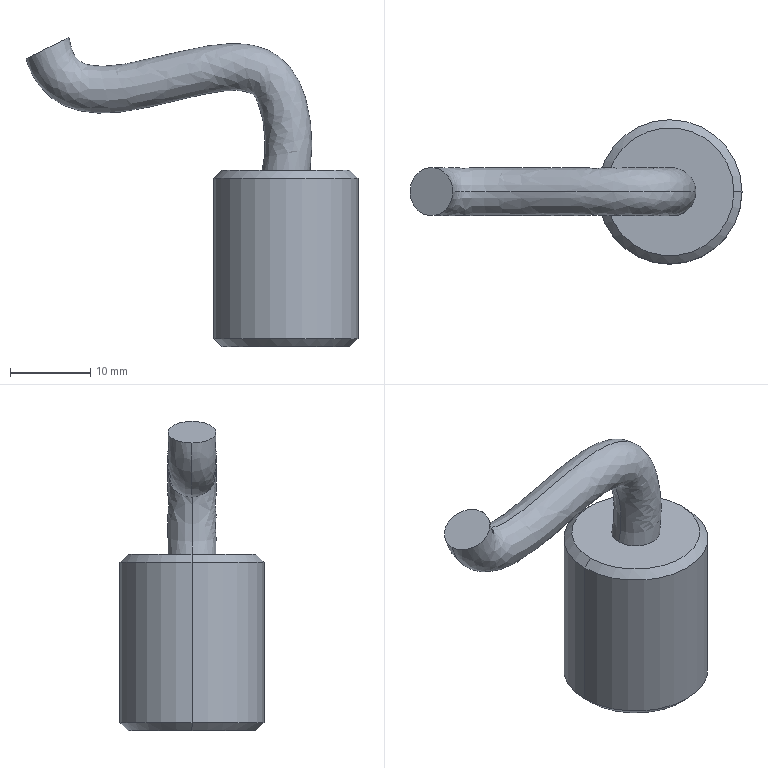Part | SolidWorks | features Chamfer 1, Extrusion 1, Sweep 1 | 1 solid | 11 faces | box 41.439 x 18 x 38.614 mm | volume 6724 mm3 | cone 4 | plane 3 | spline 2 | cylinder 2 | commonest cylinder face diameters 18 x2
STEP:
#1=CARTESIAN_POINT('',(3.,0.,11.));
#2=VERTEX_POINT('',#1);
#3=CARTESIAN_POINT('',(-3.,0.,11.));
#4=VERTEX_POINT('',#3);
#5=CARTESIAN_POINT('',(0.,0.,11.));
#6=DIRECTION('',(0.,0.,1.));
#7=DIRECTION('',(1.,0.,0.));
#8=AXIS2_PLACEMENT_3D('',#5,#6,#7);
#9=CIRCLE('',#8,3.);
#10=EDGE_CURVE('',#2,#4,#9,.T.);
#11=ORIENTED_EDGE('',*,*,#10,.T.);
#12=CARTESIAN_POINT('',(-32.439,0.,24.904));
#13=VERTEX_POINT('',#12);
#14=CARTESIAN_POINT('',(-3.,0.,11.));
#15=CARTESIAN_POINT('',(-2.85,0.,11.421));
#16=CARTESIAN_POINT('',(-2.631,0.,12.544));
#17=CARTESIAN_POINT('',(-2.558,0.,14.898));
#18=CARTESIAN_POINT('',(-2.81,0.,17.258));
#19=CARTESIAN_POINT('',(-3.262,0.,18.888));
#20=CARTESIAN_POINT('',(-3.573,0.,19.598));
#21=CARTESIAN_POINT('',(-3.703,0.,19.921));
#22=CARTESIAN_POINT('',(-3.832,0.,20.182));
#23=CARTESIAN_POINT('',(-4.134,0.,20.515));
#24=CARTESIAN_POINT('',(-5.011,0.,20.928));
#25=CARTESIAN_POINT('',(-6.881,0.,21.08));
#26=CARTESIAN_POINT('',(-10.217,0.,20.577));
#27=CARTESIAN_POINT('',(-14.463,0.,19.502));
#28=CARTESIAN_POINT('',(-19.332,0.,18.356));
#29=CARTESIAN_POINT('',(-23.167,0.,17.996));
#30=CARTESIAN_POINT('',(-25.981,0.,18.439));
#31=CARTESIAN_POINT('',(-27.667,0.,19.007));
#32=CARTESIAN_POINT('',(-29.133,0.,19.872));
#33=CARTESIAN_POINT('',(-30.31,0.,20.94));
#34=CARTESIAN_POINT('',(-31.207,0.,22.094));
#35=CARTESIAN_POINT('',(-31.928,0.,23.416));
#36=CARTESIAN_POINT('',(-32.28,0.,24.389));
#37=CARTESIAN_POINT('',(-32.439,0.,24.904));
#38=B_SPLINE_CURVE_WITH_KNOTS('',3,(#14,#15,#16,#17,#18,#19,#20,#21,#22,#23,#24,#25,#26,#27,#28,#29,#30,#31,#32,#33,#34,#35,#36,#37),.UNSPECIFIED.,.F.,.F.,(4,1,1,1,1,1,1,1,1,1,1,1,1,1,1,1,1,1,1,1,1,4),(0.,0.0625,0.125,0.1875,0.25,0.2852,0.2991,0.3203,0.3555,0.3906,0.4609,0.5313,0.625,0.7188,0.8125,0.8437,0.875,0.9063,0.9297,0.9531,0.9766,1.),.UNSPECIFIED.);
#39=EDGE_CURVE('',#4,#13,#38,.T.);
#40=ORIENTED_EDGE('',*,*,#39,.T.);
#41=CARTESIAN_POINT('',(-27.086,0.,27.614));
#42=VERTEX_POINT('',#41);
#43=CARTESIAN_POINT('',(-29.762,0.,26.259));
#44=DIRECTION('',(0.4517,0.,-0.8922));
#45=DIRECTION('',(-0.8922,0.,-0.4517));
#46=AXIS2_PLACEMENT_3D('',#43,#44,#45);
#47=CIRCLE('',#46,3.);
#48=EDGE_CURVE('',#13,#42,#47,.T.);
#49=ORIENTED_EDGE('',*,*,#48,.T.);
#50=CARTESIAN_POINT('',(3.,0.,11.));
#51=CARTESIAN_POINT('',(3.127,0.,11.782));
#52=CARTESIAN_POINT('',(3.302,0.,13.63));
#53=CARTESIAN_POINT('',(3.187,0.,16.671));
#54=CARTESIAN_POINT('',(2.615,0.,19.895));
#55=CARTESIAN_POINT('',(1.565,0.,22.549));
#56=CARTESIAN_POINT('',(0.3239,0.,24.212));
#57=CARTESIAN_POINT('',(-0.6963,0.,25.127));
#58=CARTESIAN_POINT('',(-1.844,0.,25.902));
#59=CARTESIAN_POINT('',(-3.45,0.,26.527));
#60=CARTESIAN_POINT('',(-5.923,0.,26.93));
#61=CARTESIAN_POINT('',(-8.914,0.,26.745));
#62=CARTESIAN_POINT('',(-12.881,0.,25.959));
#63=CARTESIAN_POINT('',(-17.232,0.,24.825));
#64=CARTESIAN_POINT('',(-21.638,0.,23.911));
#65=CARTESIAN_POINT('',(-24.307,0.,23.981));
#66=CARTESIAN_POINT('',(-25.501,0.,24.453));
#67=CARTESIAN_POINT('',(-25.999,0.,24.819));
#68=CARTESIAN_POINT('',(-26.304,0.,25.21));
#69=CARTESIAN_POINT('',(-26.531,0.,25.637));
#70=CARTESIAN_POINT('',(-26.728,0.,26.122));
#71=CARTESIAN_POINT('',(-26.917,0.,26.754));
#72=CARTESIAN_POINT('',(-27.041,0.,27.308));
#73=CARTESIAN_POINT('',(-27.086,0.,27.614));
#74=B_SPLINE_CURVE_WITH_KNOTS('',3,(#50,#51,#52,#53,#54,#55,#56,#57,#58,#59,#60,#61,#62,#63,#64,#65,#66,#67,#68,#69,#70,#71,#72,#73),.UNSPECIFIED.,.F.,.F.,(4,1,1,1,1,1,1,1,1,1,1,1,1,1,1,1,1,1,1,1,1,4),(0.,0.0625,0.125,0.1875,0.25,0.2852,0.2991,0.3203,0.3555,0.3906,0.4609,0.5313,0.625,0.7188,0.8125,0.8437,0.875,0.9063,0.9297,0.9531,0.9766,1.),.UNSPECIFIED.);
#75=EDGE_CURVE('',#2,#42,#74,.T.);
#76=ORIENTED_EDGE('',*,*,#75,.F.);
#77=EDGE_LOOP('',(#11,#40,#49,#76));
#78=FACE_OUTER_BOUND('',#77,.T.);
#79=CARTESIAN_POINT('',(3.,0.,11.));
#80=CARTESIAN_POINT('',(3.127,0.,11.782));
#81=CARTESIAN_POINT('',(3.302,0.,13.63));
#82=CARTESIAN_POINT('',(3.187,0.,16.671));
#83=CARTESIAN_POINT('',(2.615,0.,19.895));
#84=CARTESIAN_POINT('',(1.565,0.,22.549));
#85=CARTESIAN_POINT('',(0.3239,0.,24.212));
#86=CARTESIAN_POINT('',(-0.6963,0.,25.127));
#87=CARTESIAN_POINT('',(-1.844,0.,25.902));
#88=CARTESIAN_POINT('',(-3.45,0.,26.527));
#89=CARTESIAN_POINT('',(-5.923,0.,26.93));
#90=CARTESIAN_POINT('',(-8.914,0.,26.745));
#91=CARTESIAN_POINT('',(-12.881,0.,25.959));
#92=CARTESIAN_POINT('',(-17.232,0.,24.825));
#93=CARTESIAN_POINT('',(-21.638,0.,23.911));
#94=CARTESIAN_POINT('',(-24.307,0.,23.981));
#95=CARTESIAN_POINT('',(-25.501,0.,24.453));
#96=CARTESIAN_POINT('',(-25.999,0.,24.819));
#97=CARTESIAN_POINT('',(-26.304,0.,25.21));
#98=CARTESIAN_POINT('',(-26.531,0.,25.637));
#99=CARTESIAN_POINT('',(-26.728,0.,26.122));
#100=CARTESIAN_POINT('',(-26.917,0.,26.754));
#101=CARTESIAN_POINT('',(-27.041,0.,27.308));
#102=CARTESIAN_POINT('',(-27.086,0.,27.614));
#103=CARTESIAN_POINT('',(3.,6.,11.));
#104=CARTESIAN_POINT('',(3.127,6.,11.782));
#105=CARTESIAN_POINT('',(3.302,6.,13.63));
#106=CARTESIAN_POINT('',(3.187,6.,16.671));
#107=CARTESIAN_POINT('',(2.615,6.,19.895));
#108=CARTESIAN_POINT('',(1.565,6.,22.549));
#109=CARTESIAN_POINT('',(0.3239,6.,24.212));
#110=CARTESIAN_POINT('',(-0.6963,6.,25.127));
#111=CARTESIAN_POINT('',(-1.844,6.,25.902));
#112=CARTESIAN_POINT('',(-3.45,6.,26.527));
#113=CARTESIAN_POINT('',(-5.923,6.,26.93));
#114=CARTESIAN_POINT('',(-8.914,6.,26.745));
#115=CARTESIAN_POINT('',(-12.881,6.,25.959));
#116=CARTESIAN_POINT('',(-17.232,6.,24.825));
#117=CARTESIAN_POINT('',(-21.638,6.,23.911));
#118=CARTESIAN_POINT('',(-24.307,6.,23.981));
#119=CARTESIAN_POINT('',(-25.501,6.,24.453));
#120=CARTESIAN_POINT('',(-25.999,6.,24.819));
#121=CARTESIAN_POINT('',(-26.304,6.,25.21));
#122=CARTESIAN_POINT('',(-26.531,6.,25.637));
#123=CARTESIAN_POINT('',(-26.728,6.,26.122));
#124=CARTESIAN_POINT('',(-26.917,6.,26.754));
#125=CARTESIAN_POINT('',(-27.041,6.,27.308));
#126=CARTESIAN_POINT('',(-27.086,6.,27.614));
#127=CARTESIAN_POINT('',(-3.,6.,11.));
#128=CARTESIAN_POINT('',(-2.85,6.,11.421));
#129=CARTESIAN_POINT('',(-2.631,6.,12.544));
#130=CARTESIAN_POINT('',(-2.558,6.,14.898));
#131=CARTESIAN_POINT('',(-2.81,6.,17.258));
#132=CARTESIAN_POINT('',(-3.262,6.,18.888));
#133=CARTESIAN_POINT('',(-3.573,6.,19.598));
#134=CARTESIAN_POINT('',(-3.703,6.,19.921));
#135=CARTESIAN_POINT('',(-3.832,6.,20.182));
#136=CARTESIAN_POINT('',(-4.134,6.,20.515));
#137=CARTESIAN_POINT('',(-5.011,6.,20.928));
#138=CARTESIAN_POINT('',(-6.881,6.,21.08));
#139=CARTESIAN_POINT('',(-10.217,6.,20.577));
#140=CARTESIAN_POINT('',(-14.463,6.,19.502));
#141=CARTESIAN_POINT('',(-19.332,6.,18.356));
#142=CARTESIAN_POINT('',(-23.167,6.,17.996));
#143=CARTESIAN_POINT('',(-25.981,6.,18.439));
#144=CARTESIAN_POINT('',(-27.667,6.,19.007));
#145=CARTESIAN_POINT('',(-29.133,6.,19.872));
#146=CARTESIAN_POINT('',(-30.31,6.,20.94));
#147=CARTESIAN_POINT('',(-31.207,6.,22.094));
#148=CARTESIAN_POINT('',(-31.928,6.,23.416));
#149=CARTESIAN_POINT('',(-32.28,6.,24.389));
#150=CARTESIAN_POINT('',(-32.439,6.,24.904));
#151=CARTESIAN_POINT('',(-3.,0.,11.));
#152=CARTESIAN_POINT('',(-2.85,0.,11.421));
#153=CARTESIAN_POINT('',(-2.631,0.,12.544));
#154=CARTESIAN_POINT('',(-2.558,0.,14.898));
#155=CARTESIAN_POINT('',(-2.81,0.,17.258));
#156=CARTESIAN_POINT('',(-3.262,0.,18.888));
#157=CARTESIAN_POINT('',(-3.573,0.,19.598));
#158=CARTESIAN_POINT('',(-3.703,0.,19.921));
#159=CARTESIAN_POINT('',(-3.832,0.,20.182));
#160=CARTESIAN_POINT('',(-4.134,0.,20.515));
#161=CARTESIAN_POINT('',(-5.011,0.,20.928));
#162=CARTESIAN_POINT('',(-6.881,0.,21.08));
#163=CARTESIAN_POINT('',(-10.217,0.,20.577));
#164=CARTESIAN_POINT('',(-14.463,0.,19.502));
#165=CARTESIAN_POINT('',(-19.332,0.,18.356));
#166=CARTESIAN_POINT('',(-23.167,0.,17.996));
#167=CARTESIAN_POINT('',(-25.981,0.,18.439));
#168=CARTESIAN_POINT('',(-27.667,0.,19.007));
#169=CARTESIAN_POINT('',(-29.133,0.,19.872));
#170=CARTESIAN_POINT('',(-30.31,0.,20.94));
#171=CARTESIAN_POINT('',(-31.207,0.,22.094));
#172=CARTESIAN_POINT('',(-31.928,0.,23.416));
#173=CARTESIAN_POINT('',(-32.28,0.,24.389));
#174=CARTESIAN_POINT('',(-32.439,0.,24.904));
#175=CARTESIAN_POINT('',(-3.,-6.,11.));
#176=CARTESIAN_POINT('',(-2.85,-6.,11.421));
#177=CARTESIAN_POINT('',(-2.631,-6.,12.544));
#178=CARTESIAN_POINT('',(-2.558,-6.,14.898));
#179=CARTESIAN_POINT('',(-2.81,-6.,17.258));
#180=CARTESIAN_POINT('',(-3.262,-6.,18.888));
#181=CARTESIAN_POINT('',(-3.573,-6.,19.598));
#182=CARTESIAN_POINT('',(-3.703,-6.,19.921));
#183=CARTESIAN_POINT('',(-3.832,-6.,20.182));
#184=CARTESIAN_POINT('',(-4.134,-6.,20.515));
#185=CARTESIAN_POINT('',(-5.011,-6.,20.928));
#186=CARTESIAN_POINT('',(-6.881,-6.,21.08));
#187=CARTESIAN_POINT('',(-10.217,-6.,20.577));
#188=CARTESIAN_POINT('',(-14.463,-6.,19.502));
#189=CARTESIAN_POINT('',(-19.332,-6.,18.356));
#190=CARTESIAN_POINT('',(-23.167,-6.,17.996));
#191=CARTESIAN_POINT('',(-25.981,-6.,18.439));
#192=CARTESIAN_POINT('',(-27.667,-6.,19.007));
#193=CARTESIAN_POINT('',(-29.133,-6.,19.872));
#194=CARTESIAN_POINT('',(-30.31,-6.,20.94));
#195=CARTESIAN_POINT('',(-31.207,-6.,22.094));
#196=CARTESIAN_POINT('',(-31.928,-6.,23.416));
#197=CARTESIAN_POINT('',(-32.28,-6.,24.389));
#198=CARTESIAN_POINT('',(-32.439,-6.,24.904));
#199=CARTESIAN_POINT('',(3.,-6.,11.));
#200=CARTESIAN_POINT('',(3.127,-6.,11.782));
#201=CARTESIAN_POINT('',(3.302,-6.,13.63));
#202=CARTESIAN_POINT('',(3.187,-6.,16.671));
#203=CARTESIAN_POINT('',(2.615,-6.,19.895));
#204=CARTESIAN_POINT('',(1.565,-6.,22.549));
#205=CARTESIAN_POINT('',(0.3239,-6.,24.212));
#206=CARTESIAN_POINT('',(-0.6963,-6.,25.127));
#207=CARTESIAN_POINT('',(-1.844,-6.,25.902));
#208=CARTESIAN_POINT('',(-3.45,-6.,26.527));
#209=CARTESIAN_POINT('',(-5.923,-6.,26.93));
#210=CARTESIAN_POINT('',(-8.914,-6.,26.745));
#211=CARTESIAN_POINT('',(-12.881,-6.,25.959));
#212=CARTESIAN_POINT('',(-17.232,-6.,24.825));
#213=CARTESIAN_POINT('',(-21.638,-6.,23.911));
#214=CARTESIAN_POINT('',(-24.307,-6.,23.981));
#215=CARTESIAN_POINT('',(-25.501,-6.,24.453));
#216=CARTESIAN_POINT('',(-25.999,-6.,24.819));
#217=CARTESIAN_POINT('',(-26.304,-6.,25.21));
#218=CARTESIAN_POINT('',(-26.531,-6.,25.637));
#219=CARTESIAN_POINT('',(-26.728,-6.,26.122));
#220=CARTESIAN_POINT('',(-26.917,-6.,26.754));
#221=CARTESIAN_POINT('',(-27.041,-6.,27.308));
#222=CARTESIAN_POINT('',(-27.086,-6.,27.614));
#223=CARTESIAN_POINT('',(3.,0.,11.));
#224=CARTESIAN_POINT('',(3.127,0.,11.782));
#225=CARTESIAN_POINT('',(3.302,0.,13.63));
#226=CARTESIAN_POINT('',(3.187,0.,16.671));
#227=CARTESIAN_POINT('',(2.615,0.,19.895));
#228=CARTESIAN_POINT('',(1.565,0.,22.549));
#229=CARTESIAN_POINT('',(0.3239,0.,24.212));
#230=CARTESIAN_POINT('',(-0.6963,0.,25.127));
#231=CARTESIAN_POINT('',(-1.844,0.,25.902));
#232=CARTESIAN_POINT('',(-3.45,0.,26.527));
#233=CARTESIAN_POINT('',(-5.923,0.,26.93));
#234=CARTESIAN_POINT('',(-8.914,0.,26.745));
#235=CARTESIAN_POINT('',(-12.881,0.,25.959));
#236=CARTESIAN_POINT('',(-17.232,0.,24.825));
#237=CARTESIAN_POINT('',(-21.638,0.,23.911));
#238=CARTESIAN_POINT('',(-24.307,0.,23.981));
#239=CARTESIAN_POINT('',(-25.501,0.,24.453));
#240=CARTESIAN_POINT('',(-25.999,0.,24.819));
#241=CARTESIAN_POINT('',(-26.304,0.,25.21));
#242=CARTESIAN_POINT('',(-26.531,0.,25.637));
#243=CARTESIAN_POINT('',(-26.728,0.,26.122));
#244=CARTESIAN_POINT('',(-26.917,0.,26.754));
#245=CARTESIAN_POINT('',(-27.041,0.,27.308));
#246=CARTESIAN_POINT('',(-27.086,0.,27.614));
#247=(BOUNDED_SURFACE()B_SPLINE_SURFACE(3,3,((#79,#80,#81,#82,#83,#84,#85,#86,#87,#88,#89,#90,#91,#92,#93,#94,#95,#96,#97,#98,#99,#100,#101,#102),(#103,#104,#105,#106,#107,#108,#109,#110,#111,#112,#113,#114,#115,#116,#117,#118,#119,#120,#121,#122,#123,#124,#125,#126),(#127,#128,#129,#130,#131,#132,#133,#134,#135,#136,#137,#138,#139,#140,#141,#142,#143,#144,#145,#146,#147,#148,#149,#150),(#151,#152,#153,#154,#155,#156,#157,#158,#159,#160,#161,#162,#163,#164,#165,#166,#167,#168,#169,#170,#171,#172,#173,#174),(#175,#176,#177,#178,#179,#180,#181,#182,#183,#184,#185,#186,#187,#188,#189,#190,#191,#192,#193,#194,#195,#196,#197,#198),(#199,#200,#201,#202,#203,#204,#205,#206,#207,#208,#209,#210,#211,#212,#213,#214,#215,#216,#217,#218,#219,#220,#221,#222),(#223,#224,#225,#226,#227,#228,#229,#230,#231,#232,#233,#234,#235,#236,#237,#238,#239,#240,#241,#242,#243,#244,#245,#246)),.UNSPECIFIED.,.T.,.F.,.T.)B_SPLINE_SURFACE_WITH_KNOTS((4,3,4),(4,1,1,1,1,1,1,1,1,1,1,1,1,1,1,1,1,1,1,1,1,4),(0.,0.5,1.),(0.,0.0625,0.125,0.1875,0.25,0.2852,0.2991,0.3203,0.3555,0.3906,0.4609,0.5313,0.625,0.7188,0.8125,0.8437,0.875,0.9063,0.9297,0.9531,0.9766,1.),.UNSPECIFIED.)GEOMETRIC_REPRESENTATION_ITEM()RATIONAL_B_SPLINE_SURFACE(((1.,1.,1.,1.,1.,1.,1.,1.,1.,1.,1.,1.,1.,1.,1.,1.,1.,1.,1.,1.,1.,1.,1.,1.),(0.3333,0.3333,0.3333,0.3333,0.3333,0.3333,0.3333,0.3333,0.3333,0.3333,0.3333,0.3333,0.3333,0.3333,0.3333,0.3333,0.3333,0.3333,0.3333,0.3333,0.3333,0.3333,0.3333,0.3333),(0.3333,0.3333,0.3333,0.3333,0.3333,0.3333,0.3333,0.3333,0.3333,0.3333,0.3333,0.3333,0.3333,0.3333,0.3333,0.3333,0.3333,0.3333,0.3333,0.3333,0.3333,0.3333,0.3333,0.3333),(1.,1.,1.,1.,1.,1.,1.,1.,1.,1.,1.,1.,1.,1.,1.,1.,1.,1.,1.,1.,1.,1.,1.,1.),(0.3333,0.3333,0.3333,0.3333,0.3333,0.3333,0.3333,0.3333,0.3333,0.3333,0.3333,0.3333,0.3333,0.3333,0.3333,0.3333,0.3333,0.3333,0.3333,0.3333,0.3333,0.3333,0.3333,0.3333),(0.3333,0.3333,0.3333,0.3333,0.3333,0.3333,0.3333,0.3333,0.3333,0.3333,0.3333,0.3333,0.3333,0.3333,0.3333,0.3333,0.3333,0.3333,0.3333,0.3333,0.3333,0.3333,0.3333,0.3333),(1.,1.,1.,1.,1.,1.,1.,1.,1.,1.,1.,1.,1.,1.,1.,1.,1.,1.,1.,1.,1.,1.,1.,1.)))REPRESENTATION_ITEM('')SURFACE());
#248=ADVANCED_FACE('',(#78),#247,.T.);
#249=CARTESIAN_POINT('',(8.,0.,11.));
#250=VERTEX_POINT('',#249);
#251=CARTESIAN_POINT('',(-8.,0.,11.));
#252=VERTEX_POINT('',#251);
#253=CARTESIAN_POINT('',(0.,0.,11.));
#254=DIRECTION('',(0.,0.,1.));
#255=DIRECTION('',(1.,0.,0.));
#256=AXIS2_PLACEMENT_3D('',#253,#254,#255);
#257=CIRCLE('',#256,8.);
#258=EDGE_CURVE('',#250,#252,#257,.T.);
#259=ORIENTED_EDGE('',*,*,#258,.F.);
#260=CARTESIAN_POINT('',(9.,0.,10.));
#261=VERTEX_POINT('',#260);
#262=CARTESIAN_POINT('',(8.,0.,11.));
#263=DIRECTION('',(0.7071,0.,-0.7071));
#264=VECTOR('',#263,1000.);
#265=LINE('',#262,#264);
#266=EDGE_CURVE('',#250,#261,#265,.T.);
#267=ORIENTED_EDGE('',*,*,#266,.T.);
#268=CARTESIAN_POINT('',(-9.,0.,10.));
#269=VERTEX_POINT('',#268);
#270=CARTESIAN_POINT('',(0.,0.,10.));
#271=DIRECTION('',(0.,0.,-1.));
#272=DIRECTION('',(1.,0.,0.));
#273=AXIS2_PLACEMENT_3D('',#270,#271,#272);
#274=CIRCLE('',#273,9.);
#275=EDGE_CURVE('',#269,#261,#274,.T.);
#276=ORIENTED_EDGE('',*,*,#275,.F.);
#277=CARTESIAN_POINT('',(-8.,0.,11.));
#278=DIRECTION('',(-0.7071,0.,-0.7071));
#279=VECTOR('',#278,1000.);
#280=LINE('',#277,#279);
#281=EDGE_CURVE('',#252,#269,#280,.T.);
#282=ORIENTED_EDGE('',*,*,#281,.F.);
#283=EDGE_LOOP('',(#259,#267,#276,#282));
#284=FACE_OUTER_BOUND('',#283,.T.);
#285=CARTESIAN_POINT('',(0.,0.,11.));
#286=DIRECTION('',(0.,0.,-1.));
#287=DIRECTION('',(-1.,0.,0.));
#288=AXIS2_PLACEMENT_3D('',#285,#286,#287);
#289=CONICAL_SURFACE('',#288,8.,0.7854);
#290=ADVANCED_FACE('',(#284),#289,.T.);
#291=CARTESIAN_POINT('',(-8.,0.,-11.));
#292=VERTEX_POINT('',#291);
#293=CARTESIAN_POINT('',(8.,0.,-11.));
#294=VERTEX_POINT('',#293);
#295=CARTESIAN_POINT('',(0.,0.,-11.));
#296=DIRECTION('',(0.,0.,-1.));
#297=DIRECTION('',(1.,0.,0.));
#298=AXIS2_PLACEMENT_3D('',#295,#296,#297);
#299=CIRCLE('',#298,8.);
#300=EDGE_CURVE('',#292,#294,#299,.T.);
#301=ORIENTED_EDGE('',*,*,#300,.F.);
#302=CARTESIAN_POINT('',(-9.,0.,-10.));
#303=VERTEX_POINT('',#302);
#304=CARTESIAN_POINT('',(-9.,0.,-10.));
#305=DIRECTION('',(-0.7071,0.,0.7071));
#306=VECTOR('',#305,1000.);
#307=LINE('',#304,#306);
#308=EDGE_CURVE('',#292,#303,#307,.T.);
#309=ORIENTED_EDGE('',*,*,#308,.T.);
#310=CARTESIAN_POINT('',(9.,0.,-10.));
#311=VERTEX_POINT('',#310);
#312=CARTESIAN_POINT('',(0.,0.,-10.));
#313=DIRECTION('',(0.,0.,1.));
#314=DIRECTION('',(1.,0.,0.));
#315=AXIS2_PLACEMENT_3D('',#312,#313,#314);
#316=CIRCLE('',#315,9.);
#317=EDGE_CURVE('',#311,#303,#316,.T.);
#318=ORIENTED_EDGE('',*,*,#317,.F.);
#319=CARTESIAN_POINT('',(9.,0.,-10.));
#320=DIRECTION('',(0.7071,0.,0.7071));
#321=VECTOR('',#320,1000.);
#322=LINE('',#319,#321);
#323=EDGE_CURVE('',#294,#311,#322,.T.);
#324=ORIENTED_EDGE('',*,*,#323,.F.);
#325=EDGE_LOOP('',(#301,#309,#318,#324));
#326=FACE_OUTER_BOUND('',#325,.T.);
#327=CARTESIAN_POINT('',(0.,0.,-10.));
#328=DIRECTION('',(0.,0.,1.));
#329=DIRECTION('',(1.,0.,0.));
#330=AXIS2_PLACEMENT_3D('',#327,#328,#329);
#331=CONICAL_SURFACE('',#330,9.,0.7854);
#332=ADVANCED_FACE('',(#326),#331,.T.);
#333=ORIENTED_EDGE('',*,*,#275,.T.);
#334=CARTESIAN_POINT('',(9.,0.,11.));
#335=DIRECTION('',(0.,0.,-1.));
#336=VECTOR('',#335,1000.);
#337=LINE('',#334,#336);
#338=EDGE_CURVE('',#261,#311,#337,.T.);
#339=ORIENTED_EDGE('',*,*,#338,.T.);
#340=ORIENTED_EDGE('',*,*,#317,.T.);
#341=CARTESIAN_POINT('',(-9.,0.,11.));
#342=DIRECTION('',(0.,0.,-1.));
#343=VECTOR('',#342,1000.);
#344=LINE('',#341,#343);
#345=EDGE_CURVE('',#269,#303,#344,.T.);
#346=ORIENTED_EDGE('',*,*,#345,.F.);
#347=EDGE_LOOP('',(#333,#339,#340,#346));
#348=FACE_OUTER_BOUND('',#347,.T.);
#349=CARTESIAN_POINT('',(0.,0.,11.));
#350=DIRECTION('',(0.,0.,-1.));
#351=DIRECTION('',(-1.,0.,0.));
#352=AXIS2_PLACEMENT_3D('',#349,#350,#351);
#353=CYLINDRICAL_SURFACE('',#352,9.);
#354=ADVANCED_FACE('',(#348),#353,.T.);
#355=ORIENTED_EDGE('',*,*,#338,.F.);
#356=CARTESIAN_POINT('',(0.,0.,10.));
#357=DIRECTION('',(0.,0.,-1.));
#358=DIRECTION('',(1.,0.,0.));
#359=AXIS2_PLACEMENT_3D('',#356,#357,#358);
#360=CIRCLE('',#359,9.);
#361=EDGE_CURVE('',#261,#269,#360,.T.);
#362=ORIENTED_EDGE('',*,*,#361,.T.);
#363=ORIENTED_EDGE('',*,*,#345,.T.);
#364=CARTESIAN_POINT('',(0.,0.,-10.));
#365=DIRECTION('',(0.,0.,1.));
#366=DIRECTION('',(1.,0.,0.));
#367=AXIS2_PLACEMENT_3D('',#364,#365,#366);
#368=CIRCLE('',#367,9.);
#369=EDGE_CURVE('',#303,#311,#368,.T.);
#370=ORIENTED_EDGE('',*,*,#369,.T.);
#371=EDGE_LOOP('',(#355,#362,#363,#370));
#372=FACE_OUTER_BOUND('',#371,.T.);
#373=CARTESIAN_POINT('',(0.,0.,11.));
#374=DIRECTION('',(0.,0.,-1.));
#375=DIRECTION('',(-1.,0.,0.));
#376=AXIS2_PLACEMENT_3D('',#373,#374,#375);
#377=CYLINDRICAL_SURFACE('',#376,9.);
#378=ADVANCED_FACE('',(#372),#377,.T.);
#379=ORIENTED_EDGE('',*,*,#10,.F.);
#380=CARTESIAN_POINT('',(0.,0.,11.));
#381=DIRECTION('',(0.,0.,1.));
#382=DIRECTION('',(1.,0.,0.));
#383=AXIS2_PLACEMENT_3D('',#380,#381,#382);
#384=CIRCLE('',#383,3.);
#385=EDGE_CURVE('',#4,#2,#384,.T.);
#386=ORIENTED_EDGE('',*,*,#385,.F.);
#387=EDGE_LOOP('',(#379,#386));
#388=FACE_BOUND('',#387,.T.);
#389=CARTESIAN_POINT('',(0.,0.,11.));
#390=DIRECTION('',(0.,0.,1.));
#391=DIRECTION('',(1.,0.,0.));
#392=AXIS2_PLACEMENT_3D('',#389,#390,#391);
#393=CIRCLE('',#392,8.);
#394=EDGE_CURVE('',#252,#250,#393,.T.);
#395=ORIENTED_EDGE('',*,*,#394,.T.);
#396=ORIENTED_EDGE('',*,*,#258,.T.);
#397=EDGE_LOOP('',(#395,#396));
#398=FACE_OUTER_BOUND('',#397,.T.);
#399=CARTESIAN_POINT('',(0.,0.,11.));
#400=DIRECTION('',(0.,0.,1.));
#401=DIRECTION('',(1.,0.,0.));
#402=AXIS2_PLACEMENT_3D('',#399,#400,#401);
#403=PLANE('',#402);
#404=ADVANCED_FACE('',(#388,#398),#403,.T.);
#405=CARTESIAN_POINT('',(0.,0.,-11.));
#406=DIRECTION('',(0.,0.,-1.));
#407=DIRECTION('',(1.,0.,0.));
#408=AXIS2_PLACEMENT_3D('',#405,#406,#407);
#409=CIRCLE('',#408,8.);
#410=EDGE_CURVE('',#294,#292,#409,.T.);
#411=ORIENTED_EDGE('',*,*,#410,.T.);
#412=ORIENTED_EDGE('',*,*,#300,.T.);
#413=EDGE_LOOP('',(#411,#412));
#414=FACE_OUTER_BOUND('',#413,.T.);
#415=CARTESIAN_POINT('',(0.,0.,-11.));
#416=DIRECTION('',(0.,0.,1.));
#417=DIRECTION('',(1.,0.,0.));
#418=AXIS2_PLACEMENT_3D('',#415,#416,#417);
#419=PLANE('',#418);
#420=ADVANCED_FACE('',(#414),#419,.F.);
#421=ORIENTED_EDGE('',*,*,#308,.F.);
#422=ORIENTED_EDGE('',*,*,#410,.F.);
#423=ORIENTED_EDGE('',*,*,#323,.T.);
#424=ORIENTED_EDGE('',*,*,#369,.F.);
#425=EDGE_LOOP('',(#421,#422,#423,#424));
#426=FACE_OUTER_BOUND('',#425,.T.);
#427=CARTESIAN_POINT('',(0.,0.,-10.));
#428=DIRECTION('',(0.,0.,1.));
#429=DIRECTION('',(1.,0.,0.));
#430=AXIS2_PLACEMENT_3D('',#427,#428,#429);
#431=CONICAL_SURFACE('',#430,9.,0.7854);
#432=ADVANCED_FACE('',(#426),#431,.T.);
#433=ORIENTED_EDGE('',*,*,#266,.F.);
#434=ORIENTED_EDGE('',*,*,#394,.F.);
#435=ORIENTED_EDGE('',*,*,#281,.T.);
#436=ORIENTED_EDGE('',*,*,#361,.F.);
#437=EDGE_LOOP('',(#433,#434,#435,#436));
#438=FACE_OUTER_BOUND('',#437,.T.);
#439=CARTESIAN_POINT('',(0.,0.,11.));
#440=DIRECTION('',(0.,0.,-1.));
#441=DIRECTION('',(-1.,0.,0.));
#442=AXIS2_PLACEMENT_3D('',#439,#440,#441);
#443=CONICAL_SURFACE('',#442,8.,0.7854);
#444=ADVANCED_FACE('',(#438),#443,.T.);
#445=ORIENTED_EDGE('',*,*,#39,.F.);
#446=ORIENTED_EDGE('',*,*,#385,.T.);
#447=ORIENTED_EDGE('',*,*,#75,.T.);
#448=CARTESIAN_POINT('',(-29.762,0.,26.259));
#449=DIRECTION('',(0.4517,0.,-0.8922));
#450=DIRECTION('',(-0.8922,0.,-0.4517));
#451=AXIS2_PLACEMENT_3D('',#448,#449,#450);
#452=CIRCLE('',#451,3.);
#453=EDGE_CURVE('',#42,#13,#452,.T.);
#454=ORIENTED_EDGE('',*,*,#453,.T.);
#455=EDGE_LOOP('',(#445,#446,#447,#454));
#456=FACE_OUTER_BOUND('',#455,.T.);
#457=CARTESIAN_POINT('',(3.,0.,11.));
#458=CARTESIAN_POINT('',(3.127,0.,11.782));
#459=CARTESIAN_POINT('',(3.302,0.,13.63));
#460=CARTESIAN_POINT('',(3.187,0.,16.671));
#461=CARTESIAN_POINT('',(2.615,0.,19.895));
#462=CARTESIAN_POINT('',(1.565,0.,22.549));
#463=CARTESIAN_POINT('',(0.3239,0.,24.212));
#464=CARTESIAN_POINT('',(-0.6963,0.,25.127));
#465=CARTESIAN_POINT('',(-1.844,0.,25.902));
#466=CARTESIAN_POINT('',(-3.45,0.,26.527));
#467=CARTESIAN_POINT('',(-5.923,0.,26.93));
#468=CARTESIAN_POINT('',(-8.914,0.,26.745));
#469=CARTESIAN_POINT('',(-12.881,0.,25.959));
#470=CARTESIAN_POINT('',(-17.232,0.,24.825));
#471=CARTESIAN_POINT('',(-21.638,0.,23.911));
#472=CARTESIAN_POINT('',(-24.307,0.,23.981));
#473=CARTESIAN_POINT('',(-25.501,0.,24.453));
#474=CARTESIAN_POINT('',(-25.999,0.,24.819));
#475=CARTESIAN_POINT('',(-26.304,0.,25.21));
#476=CARTESIAN_POINT('',(-26.531,0.,25.637));
#477=CARTESIAN_POINT('',(-26.728,0.,26.122));
#478=CARTESIAN_POINT('',(-26.917,0.,26.754));
#479=CARTESIAN_POINT('',(-27.041,0.,27.308));
#480=CARTESIAN_POINT('',(-27.086,0.,27.614));
#481=CARTESIAN_POINT('',(3.,6.,11.));
#482=CARTESIAN_POINT('',(3.127,6.,11.782));
#483=CARTESIAN_POINT('',(3.302,6.,13.63));
#484=CARTESIAN_POINT('',(3.187,6.,16.671));
#485=CARTESIAN_POINT('',(2.615,6.,19.895));
#486=CARTESIAN_POINT('',(1.565,6.,22.549));
#487=CARTESIAN_POINT('',(0.3239,6.,24.212));
#488=CARTESIAN_POINT('',(-0.6963,6.,25.127));
#489=CARTESIAN_POINT('',(-1.844,6.,25.902));
#490=CARTESIAN_POINT('',(-3.45,6.,26.527));
#491=CARTESIAN_POINT('',(-5.923,6.,26.93));
#492=CARTESIAN_POINT('',(-8.914,6.,26.745));
#493=CARTESIAN_POINT('',(-12.881,6.,25.959));
#494=CARTESIAN_POINT('',(-17.232,6.,24.825));
#495=CARTESIAN_POINT('',(-21.638,6.,23.911));
#496=CARTESIAN_POINT('',(-24.307,6.,23.981));
#497=CARTESIAN_POINT('',(-25.501,6.,24.453));
#498=CARTESIAN_POINT('',(-25.999,6.,24.819));
#499=CARTESIAN_POINT('',(-26.304,6.,25.21));
#500=CARTESIAN_POINT('',(-26.531,6.,25.637));
#501=CARTESIAN_POINT('',(-26.728,6.,26.122));
#502=CARTESIAN_POINT('',(-26.917,6.,26.754));
#503=CARTESIAN_POINT('',(-27.041,6.,27.308));
#504=CARTESIAN_POINT('',(-27.086,6.,27.614));
#505=CARTESIAN_POINT('',(-3.,6.,11.));
#506=CARTESIAN_POINT('',(-2.85,6.,11.421));
#507=CARTESIAN_POINT('',(-2.631,6.,12.544));
#508=CARTESIAN_POINT('',(-2.558,6.,14.898));
#509=CARTESIAN_POINT('',(-2.81,6.,17.258));
#510=CARTESIAN_POINT('',(-3.262,6.,18.888));
#511=CARTESIAN_POINT('',(-3.573,6.,19.598));
#512=CARTESIAN_POINT('',(-3.703,6.,19.921));
#513=CARTESIAN_POINT('',(-3.832,6.,20.182));
#514=CARTESIAN_POINT('',(-4.134,6.,20.515));
#515=CARTESIAN_POINT('',(-5.011,6.,20.928));
#516=CARTESIAN_POINT('',(-6.881,6.,21.08));
#517=CARTESIAN_POINT('',(-10.217,6.,20.577));
#518=CARTESIAN_POINT('',(-14.463,6.,19.502));
#519=CARTESIAN_POINT('',(-19.332,6.,18.356));
#520=CARTESIAN_POINT('',(-23.167,6.,17.996));
#521=CARTESIAN_POINT('',(-25.981,6.,18.439));
#522=CARTESIAN_POINT('',(-27.667,6.,19.007));
#523=CARTESIAN_POINT('',(-29.133,6.,19.872));
#524=CARTESIAN_POINT('',(-30.31,6.,20.94));
#525=CARTESIAN_POINT('',(-31.207,6.,22.094));
#526=CARTESIAN_POINT('',(-31.928,6.,23.416));
#527=CARTESIAN_POINT('',(-32.28,6.,24.389));
#528=CARTESIAN_POINT('',(-32.439,6.,24.904));
#529=CARTESIAN_POINT('',(-3.,0.,11.));
#530=CARTESIAN_POINT('',(-2.85,0.,11.421));
#531=CARTESIAN_POINT('',(-2.631,0.,12.544));
#532=CARTESIAN_POINT('',(-2.558,0.,14.898));
#533=CARTESIAN_POINT('',(-2.81,0.,17.258));
#534=CARTESIAN_POINT('',(-3.262,0.,18.888));
#535=CARTESIAN_POINT('',(-3.573,0.,19.598));
#536=CARTESIAN_POINT('',(-3.703,0.,19.921));
#537=CARTESIAN_POINT('',(-3.832,0.,20.182));
#538=CARTESIAN_POINT('',(-4.134,0.,20.515));
#539=CARTESIAN_POINT('',(-5.011,0.,20.928));
#540=CARTESIAN_POINT('',(-6.881,0.,21.08));
#541=CARTESIAN_POINT('',(-10.217,0.,20.577));
#542=CARTESIAN_POINT('',(-14.463,0.,19.502));
#543=CARTESIAN_POINT('',(-19.332,0.,18.356));
#544=CARTESIAN_POINT('',(-23.167,0.,17.996));
#545=CARTESIAN_POINT('',(-25.981,0.,18.439));
#546=CARTESIAN_POINT('',(-27.667,0.,19.007));
#547=CARTESIAN_POINT('',(-29.133,0.,19.872));
#548=CARTESIAN_POINT('',(-30.31,0.,20.94));
#549=CARTESIAN_POINT('',(-31.207,0.,22.094));
#550=CARTESIAN_POINT('',(-31.928,0.,23.416));
#551=CARTESIAN_POINT('',(-32.28,0.,24.389));
#552=CARTESIAN_POINT('',(-32.439,0.,24.904));
#553=CARTESIAN_POINT('',(-3.,-6.,11.));
#554=CARTESIAN_POINT('',(-2.85,-6.,11.421));
#555=CARTESIAN_POINT('',(-2.631,-6.,12.544));
#556=CARTESIAN_POINT('',(-2.558,-6.,14.898));
#557=CARTESIAN_POINT('',(-2.81,-6.,17.258));
#558=CARTESIAN_POINT('',(-3.262,-6.,18.888));
#559=CARTESIAN_POINT('',(-3.573,-6.,19.598));
#560=CARTESIAN_POINT('',(-3.703,-6.,19.921));
#561=CARTESIAN_POINT('',(-3.832,-6.,20.182));
#562=CARTESIAN_POINT('',(-4.134,-6.,20.515));
#563=CARTESIAN_POINT('',(-5.011,-6.,20.928));
#564=CARTESIAN_POINT('',(-6.881,-6.,21.08));
#565=CARTESIAN_POINT('',(-10.217,-6.,20.577));
#566=CARTESIAN_POINT('',(-14.463,-6.,19.502));
#567=CARTESIAN_POINT('',(-19.332,-6.,18.356));
#568=CARTESIAN_POINT('',(-23.167,-6.,17.996));
#569=CARTESIAN_POINT('',(-25.981,-6.,18.439));
#570=CARTESIAN_POINT('',(-27.667,-6.,19.007));
#571=CARTESIAN_POINT('',(-29.133,-6.,19.872));
#572=CARTESIAN_POINT('',(-30.31,-6.,20.94));
#573=CARTESIAN_POINT('',(-31.207,-6.,22.094));
#574=CARTESIAN_POINT('',(-31.928,-6.,23.416));
#575=CARTESIAN_POINT('',(-32.28,-6.,24.389));
#576=CARTESIAN_POINT('',(-32.439,-6.,24.904));
#577=CARTESIAN_POINT('',(3.,-6.,11.));
#578=CARTESIAN_POINT('',(3.127,-6.,11.782));
#579=CARTESIAN_POINT('',(3.302,-6.,13.63));
#580=CARTESIAN_POINT('',(3.187,-6.,16.671));
#581=CARTESIAN_POINT('',(2.615,-6.,19.895));
#582=CARTESIAN_POINT('',(1.565,-6.,22.549));
#583=CARTESIAN_POINT('',(0.3239,-6.,24.212));
#584=CARTESIAN_POINT('',(-0.6963,-6.,25.127));
#585=CARTESIAN_POINT('',(-1.844,-6.,25.902));
#586=CARTESIAN_POINT('',(-3.45,-6.,26.527));
#587=CARTESIAN_POINT('',(-5.923,-6.,26.93));
#588=CARTESIAN_POINT('',(-8.914,-6.,26.745));
#589=CARTESIAN_POINT('',(-12.881,-6.,25.959));
#590=CARTESIAN_POINT('',(-17.232,-6.,24.825));
#591=CARTESIAN_POINT('',(-21.638,-6.,23.911));
#592=CARTESIAN_POINT('',(-24.307,-6.,23.981));
#593=CARTESIAN_POINT('',(-25.501,-6.,24.453));
#594=CARTESIAN_POINT('',(-25.999,-6.,24.819));
#595=CARTESIAN_POINT('',(-26.304,-6.,25.21));
#596=CARTESIAN_POINT('',(-26.531,-6.,25.637));
#597=CARTESIAN_POINT('',(-26.728,-6.,26.122));
#598=CARTESIAN_POINT('',(-26.917,-6.,26.754));
#599=CARTESIAN_POINT('',(-27.041,-6.,27.308));
#600=CARTESIAN_POINT('',(-27.086,-6.,27.614));
#601=CARTESIAN_POINT('',(3.,0.,11.));
#602=CARTESIAN_POINT('',(3.127,0.,11.782));
#603=CARTESIAN_POINT('',(3.302,0.,13.63));
#604=CARTESIAN_POINT('',(3.187,0.,16.671));
#605=CARTESIAN_POINT('',(2.615,0.,19.895));
#606=CARTESIAN_POINT('',(1.565,0.,22.549));
#607=CARTESIAN_POINT('',(0.3239,0.,24.212));
#608=CARTESIAN_POINT('',(-0.6963,0.,25.127));
#609=CARTESIAN_POINT('',(-1.844,0.,25.902));
#610=CARTESIAN_POINT('',(-3.45,0.,26.527));
#611=CARTESIAN_POINT('',(-5.923,0.,26.93));
#612=CARTESIAN_POINT('',(-8.914,0.,26.745));
#613=CARTESIAN_POINT('',(-12.881,0.,25.959));
#614=CARTESIAN_POINT('',(-17.232,0.,24.825));
#615=CARTESIAN_POINT('',(-21.638,0.,23.911));
#616=CARTESIAN_POINT('',(-24.307,0.,23.981));
#617=CARTESIAN_POINT('',(-25.501,0.,24.453));
#618=CARTESIAN_POINT('',(-25.999,0.,24.819));
#619=CARTESIAN_POINT('',(-26.304,0.,25.21));
#620=CARTESIAN_POINT('',(-26.531,0.,25.637));
#621=CARTESIAN_POINT('',(-26.728,0.,26.122));
#622=CARTESIAN_POINT('',(-26.917,0.,26.754));
#623=CARTESIAN_POINT('',(-27.041,0.,27.308));
#624=CARTESIAN_POINT('',(-27.086,0.,27.614));
#625=(BOUNDED_SURFACE()B_SPLINE_SURFACE(3,3,((#457,#458,#459,#460,#461,#462,#463,#464,#465,#466,#467,#468,#469,#470,#471,#472,#473,#474,#475,#476,#477,#478,#479,#480),(#481,#482,#483,#484,#485,#486,#487,#488,#489,#490,#491,#492,#493,#494,#495,#496,#497,#498,#499,#500,#501,#502,#503,#504),(#505,#506,#507,#508,#509,#510,#511,#512,#513,#514,#515,#516,#517,#518,#519,#520,#521,#522,#523,#524,#525,#526,#527,#528),(#529,#530,#531,#532,#533,#534,#535,#536,#537,#538,#539,#540,#541,#542,#543,#544,#545,#546,#547,#548,#549,#550,#551,#552),(#553,#554,#555,#556,#557,#558,#559,#560,#561,#562,#563,#564,#565,#566,#567,#568,#569,#570,#571,#572,#573,#574,#575,#576),(#577,#578,#579,#580,#581,#582,#583,#584,#585,#586,#587,#588,#589,#590,#591,#592,#593,#594,#595,#596,#597,#598,#599,#600),(#601,#602,#603,#604,#605,#606,#607,#608,#609,#610,#611,#612,#613,#614,#615,#616,#617,#618,#619,#620,#621,#622,#623,#624)),.UNSPECIFIED.,.T.,.F.,.F.)B_SPLINE_SURFACE_WITH_KNOTS((4,3,4),(4,1,1,1,1,1,1,1,1,1,1,1,1,1,1,1,1,1,1,1,1,4),(0.,0.5,1.),(0.,0.0625,0.125,0.1875,0.25,0.2852,0.2991,0.3203,0.3555,0.3906,0.4609,0.5313,0.625,0.7188,0.8125,0.8437,0.875,0.9063,0.9297,0.9531,0.9766,1.),.UNSPECIFIED.)GEOMETRIC_REPRESENTATION_ITEM()RATIONAL_B_SPLINE_SURFACE(((1.,1.,1.,1.,1.,1.,1.,1.,1.,1.,1.,1.,1.,1.,1.,1.,1.,1.,1.,1.,1.,1.,1.,1.),(0.3333,0.3333,0.3333,0.3333,0.3333,0.3333,0.3333,0.3333,0.3333,0.3333,0.3333,0.3333,0.3333,0.3333,0.3333,0.3333,0.3333,0.3333,0.3333,0.3333,0.3333,0.3333,0.3333,0.3333),(0.3333,0.3333,0.3333,0.3333,0.3333,0.3333,0.3333,0.3333,0.3333,0.3333,0.3333,0.3333,0.3333,0.3333,0.3333,0.3333,0.3333,0.3333,0.3333,0.3333,0.3333,0.3333,0.3333,0.3333),(1.,1.,1.,1.,1.,1.,1.,1.,1.,1.,1.,1.,1.,1.,1.,1.,1.,1.,1.,1.,1.,1.,1.,1.),(0.3333,0.3333,0.3333,0.3333,0.3333,0.3333,0.3333,0.3333,0.3333,0.3333,0.3333,0.3333,0.3333,0.3333,0.3333,0.3333,0.3333,0.3333,0.3333,0.3333,0.3333,0.3333,0.3333,0.3333),(0.3333,0.3333,0.3333,0.3333,0.3333,0.3333,0.3333,0.3333,0.3333,0.3333,0.3333,0.3333,0.3333,0.3333,0.3333,0.3333,0.3333,0.3333,0.3333,0.3333,0.3333,0.3333,0.3333,0.3333),(1.,1.,1.,1.,1.,1.,1.,1.,1.,1.,1.,1.,1.,1.,1.,1.,1.,1.,1.,1.,1.,1.,1.,1.)))REPRESENTATION_ITEM('')SURFACE());
#626=ADVANCED_FACE('',(#456),#625,.T.);
#627=ORIENTED_EDGE('',*,*,#453,.F.);
#628=ORIENTED_EDGE('',*,*,#48,.F.);
#629=EDGE_LOOP('',(#627,#628));
#630=FACE_OUTER_BOUND('',#629,.T.);
#631=CARTESIAN_POINT('',(-32.439,0.,24.904));
#632=DIRECTION('',(0.4517,0.,-0.8922));
#633=DIRECTION('',(-0.8922,0.,-0.4517));
#634=AXIS2_PLACEMENT_3D('',#631,#632,#633);
#635=PLANE('',#634);
#636=ADVANCED_FACE('',(#630),#635,.F.);
#637=CLOSED_SHELL('',(#248,#290,#332,#354,#378,#404,#420,#432,#444,#626,#636));
#638=MANIFOLD_SOLID_BREP('',#637);
#639=CARTESIAN_POINT('',(0.,0.,0.));
#640=DIRECTION('',(0.,0.,1.));
#641=DIRECTION('',(1.,0.,0.));
#642=AXIS2_PLACEMENT_3D('',#639,#640,#641);
#643=(LENGTH_UNIT()NAMED_UNIT(*)SI_UNIT(.MILLI.,.METRE.));
#644=UNCERTAINTY_MEASURE_WITH_UNIT(LENGTH_MEASURE(0.00001),#643,'','');
#645=(NAMED_UNIT(*)PLANE_ANGLE_UNIT()SI_UNIT($,.RADIAN.));
#646=(NAMED_UNIT(*)SI_UNIT($,.STERADIAN.)SOLID_ANGLE_UNIT());
#647=(GEOMETRIC_REPRESENTATION_CONTEXT(3)GLOBAL_UNCERTAINTY_ASSIGNED_CONTEXT((#644))GLOBAL_UNIT_ASSIGNED_CONTEXT((#643,#645,#646))REPRESENTATION_CONTEXT('',''));
#648=ADVANCED_BREP_SHAPE_REPRESENTATION('',(#638,#642),#647);